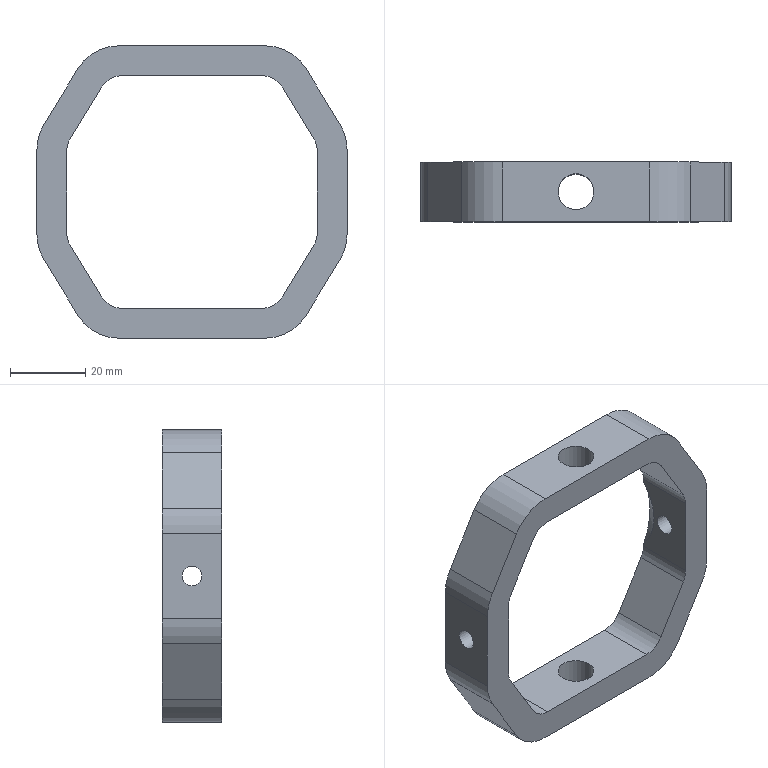Part | NX | features MG0330 trunion parts 24(gimbal) 2 | 1 solid | 40 faces | box 82.55 x 15.875 x 77.826 mm | volume 29721 mm3 | cylinder 22 | plane 18 | commonest cylinder face diameters 12.7 x8 25.4 x8 5.309 x2 9.525 x2 52.388 x2
STEP:
#1=CARTESIAN_POINT('',(33.337,-6.35,-2.654));
#2=VERTEX_POINT('',#1);
#3=CARTESIAN_POINT('',(33.337,-6.35,0.));
#4=DIRECTION('',(1.,0.,0.));
#5=DIRECTION('',(0.,0.,-1.));
#6=AXIS2_PLACEMENT_3D('',#3,#4,#5);
#7=CIRCLE('',#6,2.654);
#8=EDGE_CURVE('',#2,#2,#7,.T.);
#9=ORIENTED_EDGE('',*,*,#8,.T.);
#10=EDGE_LOOP('',(#9));
#11=FACE_BOUND('',#10,.T.);
#12=CARTESIAN_POINT('',(33.337,1.587,-10.342));
#13=VERTEX_POINT('',#12);
#14=CARTESIAN_POINT('',(33.337,1.587,-10.921));
#15=VERTEX_POINT('',#14);
#16=CARTESIAN_POINT('',(33.337,1.587,0.));
#17=DIRECTION('',(0.,0.,1.));
#18=VECTOR('',#17,1000.);
#19=LINE('',#16,#18);
#20=EDGE_CURVE('',#13,#15,#19,.F.);
#21=ORIENTED_EDGE('',*,*,#20,.T.);
#22=CARTESIAN_POINT('',(33.337,-14.287,-10.921));
#23=VERTEX_POINT('',#22);
#24=CARTESIAN_POINT('',(33.337,-14.287,-10.921));
#25=DIRECTION('',(0.,-1.,0.));
#26=VECTOR('',#25,1000.);
#27=LINE('',#24,#26);
#28=EDGE_CURVE('',#15,#23,#27,.T.);
#29=ORIENTED_EDGE('',*,*,#28,.T.);
#30=CARTESIAN_POINT('',(33.337,-14.287,10.921));
#31=VERTEX_POINT('',#30);
#32=CARTESIAN_POINT('',(33.337,-14.287,0.));
#33=DIRECTION('',(0.,0.,1.));
#34=VECTOR('',#33,1000.);
#35=LINE('',#32,#34);
#36=EDGE_CURVE('',#23,#31,#35,.T.);
#37=ORIENTED_EDGE('',*,*,#36,.T.);
#38=CARTESIAN_POINT('',(33.337,1.587,10.921));
#39=VERTEX_POINT('',#38);
#40=CARTESIAN_POINT('',(33.337,-14.287,10.921));
#41=DIRECTION('',(0.,-1.,0.));
#42=VECTOR('',#41,1000.);
#43=LINE('',#40,#42);
#44=EDGE_CURVE('',#39,#31,#43,.T.);
#45=ORIENTED_EDGE('',*,*,#44,.F.);
#46=CARTESIAN_POINT('',(33.337,1.587,10.342));
#47=VERTEX_POINT('',#46);
#48=CARTESIAN_POINT('',(33.337,1.587,0.));
#49=DIRECTION('',(0.,0.,-1.));
#50=VECTOR('',#49,1000.);
#51=LINE('',#48,#50);
#52=EDGE_CURVE('',#39,#47,#51,.T.);
#53=ORIENTED_EDGE('',*,*,#52,.T.);
#54=CARTESIAN_POINT('',(33.337,47.001,0.));
#55=DIRECTION('',(1.,0.,0.));
#56=DIRECTION('',(0.,-1.,0.));
#57=AXIS2_PLACEMENT_3D('',#54,#55,#56);
#58=ELLIPSE('',#57,49.43,26.194);
#59=EDGE_CURVE('',#13,#47,#58,.F.);
#60=ORIENTED_EDGE('',*,*,#59,.F.);
#61=EDGE_LOOP('',(#21,#29,#37,#45,#53,#60));
#62=FACE_BOUND('',#61,.T.);
#63=CARTESIAN_POINT('',(33.337,1.587,0.));
#64=DIRECTION('',(1.,0.,0.));
#65=DIRECTION('',(0.,0.,-1.));
#66=AXIS2_PLACEMENT_3D('',#63,#64,#65);
#67=PLANE('',#66);
#68=ADVANCED_FACE('',(#11,#62),#67,.F.);
#69=CARTESIAN_POINT('',(41.275,-6.35,2.654));
#70=VERTEX_POINT('',#69);
#71=CARTESIAN_POINT('',(41.275,-6.35,0.));
#72=DIRECTION('',(-1.,0.,0.));
#73=DIRECTION('',(0.,0.,1.));
#74=AXIS2_PLACEMENT_3D('',#71,#72,#73);
#75=CIRCLE('',#74,2.654);
#76=EDGE_CURVE('',#70,#70,#75,.T.);
#77=ORIENTED_EDGE('',*,*,#76,.T.);
#78=EDGE_LOOP('',(#77));
#79=FACE_BOUND('',#78,.T.);
#80=CARTESIAN_POINT('',(41.275,-14.287,11.366));
#81=VERTEX_POINT('',#80);
#82=CARTESIAN_POINT('',(41.275,-14.287,-11.366));
#83=VERTEX_POINT('',#82);
#84=CARTESIAN_POINT('',(41.275,-14.287,0.));
#85=DIRECTION('',(0.,0.,-1.));
#86=VECTOR('',#85,1000.);
#87=LINE('',#84,#86);
#88=EDGE_CURVE('',#81,#83,#87,.T.);
#89=ORIENTED_EDGE('',*,*,#88,.T.);
#90=CARTESIAN_POINT('',(41.275,1.587,-11.366));
#91=VERTEX_POINT('',#90);
#92=CARTESIAN_POINT('',(41.275,1.587,-11.366));
#93=DIRECTION('',(0.,-1.,0.));
#94=VECTOR('',#93,1000.);
#95=LINE('',#92,#94);
#96=EDGE_CURVE('',#83,#91,#95,.F.);
#97=ORIENTED_EDGE('',*,*,#96,.T.);
#98=CARTESIAN_POINT('',(41.275,1.587,11.366));
#99=VERTEX_POINT('',#98);
#100=CARTESIAN_POINT('',(41.275,1.587,0.));
#101=DIRECTION('',(0.,0.,-1.));
#102=VECTOR('',#101,1000.);
#103=LINE('',#100,#102);
#104=EDGE_CURVE('',#99,#91,#103,.T.);
#105=ORIENTED_EDGE('',*,*,#104,.F.);
#106=CARTESIAN_POINT('',(41.275,1.587,11.366));
#107=DIRECTION('',(0.,-1.,0.));
#108=VECTOR('',#107,1000.);
#109=LINE('',#106,#108);
#110=EDGE_CURVE('',#81,#99,#109,.F.);
#111=ORIENTED_EDGE('',*,*,#110,.F.);
#112=EDGE_LOOP('',(#89,#97,#105,#111));
#113=FACE_BOUND('',#112,.T.);
#114=CARTESIAN_POINT('',(41.275,1.587,0.));
#115=DIRECTION('',(-1.,0.,0.));
#116=DIRECTION('',(0.,0.,1.));
#117=AXIS2_PLACEMENT_3D('',#114,#115,#116);
#118=PLANE('',#117);
#119=ADVANCED_FACE('',(#79,#113),#118,.F.);
#120=CARTESIAN_POINT('',(39.426,1.587,-17.964));
#121=VERTEX_POINT('',#120);
#122=CARTESIAN_POINT('',(30.398,1.587,-32.811));
#123=VERTEX_POINT('',#122);
#124=CARTESIAN_POINT('',(41.275,1.587,-14.924));
#125=DIRECTION('',(-0.5196,0.,-0.8544));
#126=VECTOR('',#125,1000.);
#127=LINE('',#124,#126);
#128=EDGE_CURVE('',#121,#123,#127,.T.);
#129=ORIENTED_EDGE('',*,*,#128,.F.);
#130=CARTESIAN_POINT('',(39.426,-14.287,-17.964));
#131=VERTEX_POINT('',#130);
#132=CARTESIAN_POINT('',(39.426,1.587,-17.964));
#133=DIRECTION('',(0.,-1.,0.));
#134=VECTOR('',#133,1000.);
#135=LINE('',#132,#134);
#136=EDGE_CURVE('',#121,#131,#135,.T.);
#137=ORIENTED_EDGE('',*,*,#136,.T.);
#138=CARTESIAN_POINT('',(30.398,-14.287,-32.811));
#139=VERTEX_POINT('',#138);
#140=CARTESIAN_POINT('',(41.275,-14.287,-14.924));
#141=DIRECTION('',(-0.5196,0.,-0.8544));
#142=VECTOR('',#141,1000.);
#143=LINE('',#140,#142);
#144=EDGE_CURVE('',#131,#139,#143,.T.);
#145=ORIENTED_EDGE('',*,*,#144,.T.);
#146=CARTESIAN_POINT('',(30.398,1.587,-32.811));
#147=DIRECTION('',(0.,-1.,0.));
#148=VECTOR('',#147,1000.);
#149=LINE('',#146,#148);
#150=EDGE_CURVE('',#139,#123,#149,.F.);
#151=ORIENTED_EDGE('',*,*,#150,.T.);
#152=EDGE_LOOP('',(#129,#137,#145,#151));
#153=FACE_BOUND('',#152,.T.);
#154=CARTESIAN_POINT('',(41.275,1.587,-14.924));
#155=DIRECTION('',(-0.8544,0.,0.5196));
#156=DIRECTION('',(0.5196,0.,0.8544));
#157=AXIS2_PLACEMENT_3D('',#154,#155,#156);
#158=PLANE('',#157);
#159=ADVANCED_FACE('',(#153),#158,.F.);
#160=CARTESIAN_POINT('',(4.763,-6.35,-38.913));
#161=VERTEX_POINT('',#160);
#162=CARTESIAN_POINT('',(0.,-6.35,-38.913));
#163=DIRECTION('',(0.,0.,1.));
#164=DIRECTION('',(1.,0.,0.));
#165=AXIS2_PLACEMENT_3D('',#162,#163,#164);
#166=CIRCLE('',#165,4.763);
#167=EDGE_CURVE('',#161,#161,#166,.T.);
#168=ORIENTED_EDGE('',*,*,#167,.T.);
#169=EDGE_LOOP('',(#168));
#170=FACE_BOUND('',#169,.T.);
#171=CARTESIAN_POINT('',(19.547,1.587,-38.913));
#172=VERTEX_POINT('',#171);
#173=CARTESIAN_POINT('',(-19.547,1.587,-38.913));
#174=VERTEX_POINT('',#173);
#175=CARTESIAN_POINT('',(0.,1.587,-38.913));
#176=DIRECTION('',(-1.,0.,0.));
#177=VECTOR('',#176,1000.);
#178=LINE('',#175,#177);
#179=EDGE_CURVE('',#172,#174,#178,.T.);
#180=ORIENTED_EDGE('',*,*,#179,.F.);
#181=CARTESIAN_POINT('',(19.547,-14.287,-38.913));
#182=VERTEX_POINT('',#181);
#183=CARTESIAN_POINT('',(19.547,1.587,-38.913));
#184=DIRECTION('',(0.,-1.,0.));
#185=VECTOR('',#184,1000.);
#186=LINE('',#183,#185);
#187=EDGE_CURVE('',#172,#182,#186,.T.);
#188=ORIENTED_EDGE('',*,*,#187,.T.);
#189=CARTESIAN_POINT('',(-19.547,-14.287,-38.913));
#190=VERTEX_POINT('',#189);
#191=CARTESIAN_POINT('',(0.,-14.287,-38.913));
#192=DIRECTION('',(-1.,0.,0.));
#193=VECTOR('',#192,1000.);
#194=LINE('',#191,#193);
#195=EDGE_CURVE('',#182,#190,#194,.T.);
#196=ORIENTED_EDGE('',*,*,#195,.T.);
#197=CARTESIAN_POINT('',(-19.547,1.587,-38.913));
#198=DIRECTION('',(0.,-1.,0.));
#199=VECTOR('',#198,1000.);
#200=LINE('',#197,#199);
#201=EDGE_CURVE('',#174,#190,#200,.T.);
#202=ORIENTED_EDGE('',*,*,#201,.F.);
#203=EDGE_LOOP('',(#180,#188,#196,#202));
#204=FACE_BOUND('',#203,.T.);
#205=CARTESIAN_POINT('',(0.,1.587,-38.913));
#206=DIRECTION('',(0.,0.,1.));
#207=DIRECTION('',(1.,0.,0.));
#208=AXIS2_PLACEMENT_3D('',#205,#206,#207);
#209=PLANE('',#208);
#210=ADVANCED_FACE('',(#170,#204),#209,.F.);
#211=CARTESIAN_POINT('',(-4.763,-6.35,-30.975));
#212=VERTEX_POINT('',#211);
#213=CARTESIAN_POINT('',(0.,-6.35,-30.975));
#214=DIRECTION('',(0.,0.,-1.));
#215=DIRECTION('',(-1.,0.,0.));
#216=AXIS2_PLACEMENT_3D('',#213,#214,#215);
#217=CIRCLE('',#216,4.763);
#218=EDGE_CURVE('',#212,#212,#217,.T.);
#219=ORIENTED_EDGE('',*,*,#218,.T.);
#220=EDGE_LOOP('',(#219));
#221=FACE_BOUND('',#220,.T.);
#222=CARTESIAN_POINT('',(-18.654,-14.287,-30.975));
#223=VERTEX_POINT('',#222);
#224=CARTESIAN_POINT('',(18.654,-14.287,-30.975));
#225=VERTEX_POINT('',#224);
#226=CARTESIAN_POINT('',(0.,-14.287,-30.975));
#227=DIRECTION('',(1.,0.,0.));
#228=VECTOR('',#227,1000.);
#229=LINE('',#226,#228);
#230=EDGE_CURVE('',#223,#225,#229,.T.);
#231=ORIENTED_EDGE('',*,*,#230,.T.);
#232=CARTESIAN_POINT('',(18.654,1.587,-30.975));
#233=VERTEX_POINT('',#232);
#234=CARTESIAN_POINT('',(18.654,1.587,-30.975));
#235=DIRECTION('',(0.,-1.,0.));
#236=VECTOR('',#235,1000.);
#237=LINE('',#234,#236);
#238=EDGE_CURVE('',#225,#233,#237,.F.);
#239=ORIENTED_EDGE('',*,*,#238,.T.);
#240=CARTESIAN_POINT('',(-18.654,1.587,-30.975));
#241=VERTEX_POINT('',#240);
#242=CARTESIAN_POINT('',(0.,1.587,-30.975));
#243=DIRECTION('',(1.,0.,0.));
#244=VECTOR('',#243,1000.);
#245=LINE('',#242,#244);
#246=EDGE_CURVE('',#241,#233,#245,.T.);
#247=ORIENTED_EDGE('',*,*,#246,.F.);
#248=CARTESIAN_POINT('',(-18.654,1.587,-30.975));
#249=DIRECTION('',(0.,-1.,0.));
#250=VECTOR('',#249,1000.);
#251=LINE('',#248,#250);
#252=EDGE_CURVE('',#223,#241,#251,.F.);
#253=ORIENTED_EDGE('',*,*,#252,.F.);
#254=EDGE_LOOP('',(#231,#239,#247,#253));
#255=FACE_BOUND('',#254,.T.);
#256=CARTESIAN_POINT('',(0.,1.587,-30.975));
#257=DIRECTION('',(0.,0.,-1.));
#258=DIRECTION('',(-1.,0.,0.));
#259=AXIS2_PLACEMENT_3D('',#256,#257,#258);
#260=PLANE('',#259);
#261=ADVANCED_FACE('',(#221,#255),#260,.F.);
#262=CARTESIAN_POINT('',(24.08,1.587,-27.924));
#263=VERTEX_POINT('',#262);
#264=CARTESIAN_POINT('',(32.413,1.587,-14.22));
#265=VERTEX_POINT('',#264);
#266=CARTESIAN_POINT('',(33.337,1.587,-12.7));
#267=DIRECTION('',(0.5196,0.,0.8544));
#268=VECTOR('',#267,1000.);
#269=LINE('',#266,#268);
#270=EDGE_CURVE('',#263,#265,#269,.T.);
#271=ORIENTED_EDGE('',*,*,#270,.F.);
#272=CARTESIAN_POINT('',(24.08,-14.287,-27.924));
#273=VERTEX_POINT('',#272);
#274=CARTESIAN_POINT('',(24.08,-14.287,-27.924));
#275=DIRECTION('',(0.,-1.,0.));
#276=VECTOR('',#275,1000.);
#277=LINE('',#274,#276);
#278=EDGE_CURVE('',#263,#273,#277,.T.);
#279=ORIENTED_EDGE('',*,*,#278,.T.);
#280=CARTESIAN_POINT('',(32.413,-14.287,-14.22));
#281=VERTEX_POINT('',#280);
#282=CARTESIAN_POINT('',(33.337,-14.287,-12.7));
#283=DIRECTION('',(0.5196,0.,0.8544));
#284=VECTOR('',#283,1000.);
#285=LINE('',#282,#284);
#286=EDGE_CURVE('',#273,#281,#285,.T.);
#287=ORIENTED_EDGE('',*,*,#286,.T.);
#288=CARTESIAN_POINT('',(32.413,1.587,-14.22));
#289=DIRECTION('',(0.,-1.,0.));
#290=VECTOR('',#289,1000.);
#291=LINE('',#288,#290);
#292=EDGE_CURVE('',#281,#265,#291,.F.);
#293=ORIENTED_EDGE('',*,*,#292,.T.);
#294=EDGE_LOOP('',(#271,#279,#287,#293));
#295=FACE_BOUND('',#294,.T.);
#296=CARTESIAN_POINT('',(33.337,1.587,-12.7));
#297=DIRECTION('',(0.8544,0.,-0.5196));
#298=DIRECTION('',(-0.5196,0.,-0.8544));
#299=AXIS2_PLACEMENT_3D('',#296,#297,#298);
#300=PLANE('',#299);
#301=ADVANCED_FACE('',(#295),#300,.F.);
#302=CARTESIAN_POINT('',(-24.08,1.587,-27.924));
#303=VERTEX_POINT('',#302);
#304=CARTESIAN_POINT('',(-18.654,1.587,-24.625));
#305=DIRECTION('',(0.,1.,0.));
#306=DIRECTION('',(0.,0.,-1.));
#307=AXIS2_PLACEMENT_3D('',#304,#305,#306);
#308=CIRCLE('',#307,6.35);
#309=EDGE_CURVE('',#241,#303,#308,.T.);
#310=ORIENTED_EDGE('',*,*,#309,.F.);
#311=ORIENTED_EDGE('',*,*,#246,.T.);
#312=CARTESIAN_POINT('',(18.654,1.587,-24.625));
#313=DIRECTION('',(0.,-1.,0.));
#314=DIRECTION('',(0.,0.,-1.));
#315=AXIS2_PLACEMENT_3D('',#312,#313,#314);
#316=CIRCLE('',#315,6.35);
#317=EDGE_CURVE('',#233,#263,#316,.T.);
#318=ORIENTED_EDGE('',*,*,#317,.T.);
#319=ORIENTED_EDGE('',*,*,#270,.T.);
#320=CARTESIAN_POINT('',(26.988,1.587,-10.921));
#321=DIRECTION('',(0.,-1.,0.));
#322=DIRECTION('',(0.,0.,-1.));
#323=AXIS2_PLACEMENT_3D('',#320,#321,#322);
#324=CIRCLE('',#323,6.35);
#325=EDGE_CURVE('',#265,#15,#324,.T.);
#326=ORIENTED_EDGE('',*,*,#325,.T.);
#327=ORIENTED_EDGE('',*,*,#20,.F.);
#328=CARTESIAN_POINT('',(4.96,1.587,0.));
#329=DIRECTION('',(0.,-1.,0.));
#330=DIRECTION('',(-1.,0.,0.));
#331=AXIS2_PLACEMENT_3D('',#328,#329,#330);
#332=ELLIPSE('',#331,30.887,26.194);
#333=EDGE_CURVE('',#47,#13,#332,.F.);
#334=ORIENTED_EDGE('',*,*,#333,.F.);
#335=ORIENTED_EDGE('',*,*,#52,.F.);
#336=CARTESIAN_POINT('',(32.413,1.587,14.22));
#337=VERTEX_POINT('',#336);
#338=CARTESIAN_POINT('',(26.988,1.587,10.921));
#339=DIRECTION('',(0.,1.,0.));
#340=DIRECTION('',(0.,0.,1.));
#341=AXIS2_PLACEMENT_3D('',#338,#339,#340);
#342=CIRCLE('',#341,6.35);
#343=EDGE_CURVE('',#337,#39,#342,.T.);
#344=ORIENTED_EDGE('',*,*,#343,.F.);
#345=CARTESIAN_POINT('',(24.08,1.587,27.924));
#346=VERTEX_POINT('',#345);
#347=CARTESIAN_POINT('',(33.337,1.587,12.7));
#348=DIRECTION('',(0.5196,0.,-0.8544));
#349=VECTOR('',#348,1000.);
#350=LINE('',#347,#349);
#351=EDGE_CURVE('',#346,#337,#350,.T.);
#352=ORIENTED_EDGE('',*,*,#351,.F.);
#353=CARTESIAN_POINT('',(18.654,1.587,30.975));
#354=VERTEX_POINT('',#353);
#355=CARTESIAN_POINT('',(18.654,1.587,24.625));
#356=DIRECTION('',(0.,1.,0.));
#357=DIRECTION('',(0.,0.,1.));
#358=AXIS2_PLACEMENT_3D('',#355,#356,#357);
#359=CIRCLE('',#358,6.35);
#360=EDGE_CURVE('',#354,#346,#359,.T.);
#361=ORIENTED_EDGE('',*,*,#360,.F.);
#362=CARTESIAN_POINT('',(-18.654,1.587,30.975));
#363=VERTEX_POINT('',#362);
#364=CARTESIAN_POINT('',(0.,1.587,30.975));
#365=DIRECTION('',(1.,0.,0.));
#366=VECTOR('',#365,1000.);
#367=LINE('',#364,#366);
#368=EDGE_CURVE('',#363,#354,#367,.T.);
#369=ORIENTED_EDGE('',*,*,#368,.F.);
#370=CARTESIAN_POINT('',(-24.08,1.587,27.924));
#371=VERTEX_POINT('',#370);
#372=CARTESIAN_POINT('',(-18.654,1.587,24.625));
#373=DIRECTION('',(0.,-1.,0.));
#374=DIRECTION('',(0.,0.,1.));
#375=AXIS2_PLACEMENT_3D('',#372,#373,#374);
#376=CIRCLE('',#375,6.35);
#377=EDGE_CURVE('',#363,#371,#376,.T.);
#378=ORIENTED_EDGE('',*,*,#377,.T.);
#379=CARTESIAN_POINT('',(-32.413,1.587,14.22));
#380=VERTEX_POINT('',#379);
#381=CARTESIAN_POINT('',(-33.337,1.587,12.7));
#382=DIRECTION('',(-0.5196,0.,-0.8544));
#383=VECTOR('',#382,1000.);
#384=LINE('',#381,#383);
#385=EDGE_CURVE('',#371,#380,#384,.T.);
#386=ORIENTED_EDGE('',*,*,#385,.T.);
#387=CARTESIAN_POINT('',(-33.337,1.587,10.921));
#388=VERTEX_POINT('',#387);
#389=CARTESIAN_POINT('',(-26.988,1.587,10.921));
#390=DIRECTION('',(0.,-1.,0.));
#391=DIRECTION('',(0.,0.,1.));
#392=AXIS2_PLACEMENT_3D('',#389,#390,#391);
#393=CIRCLE('',#392,6.35);
#394=EDGE_CURVE('',#380,#388,#393,.T.);
#395=ORIENTED_EDGE('',*,*,#394,.T.);
#396=CARTESIAN_POINT('',(-33.337,1.587,10.342));
#397=VERTEX_POINT('',#396);
#398=CARTESIAN_POINT('',(-33.337,1.587,0.));
#399=DIRECTION('',(0.,0.,-1.));
#400=VECTOR('',#399,1000.);
#401=LINE('',#398,#400);
#402=EDGE_CURVE('',#388,#397,#401,.T.);
#403=ORIENTED_EDGE('',*,*,#402,.T.);
#404=CARTESIAN_POINT('',(-33.337,1.587,-10.342));
#405=VERTEX_POINT('',#404);
#406=CARTESIAN_POINT('',(-4.96,1.587,0.));
#407=DIRECTION('',(0.,1.,0.));
#408=DIRECTION('',(1.,0.,0.));
#409=AXIS2_PLACEMENT_3D('',#406,#407,#408);
#410=ELLIPSE('',#409,30.887,26.194);
#411=EDGE_CURVE('',#397,#405,#410,.F.);
#412=ORIENTED_EDGE('',*,*,#411,.T.);
#413=CARTESIAN_POINT('',(-33.337,1.587,-10.921));
#414=VERTEX_POINT('',#413);
#415=CARTESIAN_POINT('',(-33.337,1.587,0.));
#416=DIRECTION('',(0.,0.,1.));
#417=VECTOR('',#416,1000.);
#418=LINE('',#415,#417);
#419=EDGE_CURVE('',#405,#414,#418,.F.);
#420=ORIENTED_EDGE('',*,*,#419,.T.);
#421=CARTESIAN_POINT('',(-32.413,1.587,-14.22));
#422=VERTEX_POINT('',#421);
#423=CARTESIAN_POINT('',(-26.988,1.587,-10.921));
#424=DIRECTION('',(0.,1.,0.));
#425=DIRECTION('',(0.,0.,-1.));
#426=AXIS2_PLACEMENT_3D('',#423,#424,#425);
#427=CIRCLE('',#426,6.35);
#428=EDGE_CURVE('',#422,#414,#427,.T.);
#429=ORIENTED_EDGE('',*,*,#428,.F.);
#430=CARTESIAN_POINT('',(-33.337,1.587,-12.7));
#431=DIRECTION('',(-0.5196,0.,0.8544));
#432=VECTOR('',#431,1000.);
#433=LINE('',#430,#432);
#434=EDGE_CURVE('',#303,#422,#433,.T.);
#435=ORIENTED_EDGE('',*,*,#434,.F.);
#436=EDGE_LOOP('',(#310,#311,#318,#319,#326,#327,#334,#335,#344,#352,#361,#369,#378,#386,#395,#403,#412,#420,#429,#435));
#437=FACE_BOUND('',#436,.T.);
#438=ORIENTED_EDGE('',*,*,#104,.T.);
#439=CARTESIAN_POINT('',(28.575,1.587,-11.366));
#440=DIRECTION('',(0.,-1.,0.));
#441=DIRECTION('',(0.,0.,-1.));
#442=AXIS2_PLACEMENT_3D('',#439,#440,#441);
#443=CIRCLE('',#442,12.7);
#444=EDGE_CURVE('',#91,#121,#443,.F.);
#445=ORIENTED_EDGE('',*,*,#444,.T.);
#446=ORIENTED_EDGE('',*,*,#128,.T.);
#447=CARTESIAN_POINT('',(19.547,1.587,-26.213));
#448=DIRECTION('',(0.,-1.,0.));
#449=DIRECTION('',(0.,0.,-1.));
#450=AXIS2_PLACEMENT_3D('',#447,#448,#449);
#451=CIRCLE('',#450,12.7);
#452=EDGE_CURVE('',#123,#172,#451,.F.);
#453=ORIENTED_EDGE('',*,*,#452,.T.);
#454=ORIENTED_EDGE('',*,*,#179,.T.);
#455=CARTESIAN_POINT('',(-30.398,1.587,-32.811));
#456=VERTEX_POINT('',#455);
#457=CARTESIAN_POINT('',(-19.547,1.587,-26.213));
#458=DIRECTION('',(0.,1.,0.));
#459=DIRECTION('',(0.,0.,-1.));
#460=AXIS2_PLACEMENT_3D('',#457,#458,#459);
#461=CIRCLE('',#460,12.7);
#462=EDGE_CURVE('',#456,#174,#461,.F.);
#463=ORIENTED_EDGE('',*,*,#462,.F.);
#464=CARTESIAN_POINT('',(-39.426,1.587,-17.964));
#465=VERTEX_POINT('',#464);
#466=CARTESIAN_POINT('',(-41.275,1.587,-14.924));
#467=DIRECTION('',(0.5196,0.,-0.8544));
#468=VECTOR('',#467,1000.);
#469=LINE('',#466,#468);
#470=EDGE_CURVE('',#465,#456,#469,.T.);
#471=ORIENTED_EDGE('',*,*,#470,.F.);
#472=CARTESIAN_POINT('',(-41.275,1.587,-11.366));
#473=VERTEX_POINT('',#472);
#474=CARTESIAN_POINT('',(-28.575,1.587,-11.366));
#475=DIRECTION('',(0.,1.,0.));
#476=DIRECTION('',(0.,0.,-1.));
#477=AXIS2_PLACEMENT_3D('',#474,#475,#476);
#478=CIRCLE('',#477,12.7);
#479=EDGE_CURVE('',#473,#465,#478,.F.);
#480=ORIENTED_EDGE('',*,*,#479,.F.);
#481=CARTESIAN_POINT('',(-41.275,1.587,11.366));
#482=VERTEX_POINT('',#481);
#483=CARTESIAN_POINT('',(-41.275,1.587,0.));
#484=DIRECTION('',(0.,0.,-1.));
#485=VECTOR('',#484,1000.);
#486=LINE('',#483,#485);
#487=EDGE_CURVE('',#482,#473,#486,.T.);
#488=ORIENTED_EDGE('',*,*,#487,.F.);
#489=CARTESIAN_POINT('',(-39.426,1.587,17.964));
#490=VERTEX_POINT('',#489);
#491=CARTESIAN_POINT('',(-28.575,1.587,11.366));
#492=DIRECTION('',(0.,-1.,0.));
#493=DIRECTION('',(0.,0.,1.));
#494=AXIS2_PLACEMENT_3D('',#491,#492,#493);
#495=CIRCLE('',#494,12.7);
#496=EDGE_CURVE('',#482,#490,#495,.F.);
#497=ORIENTED_EDGE('',*,*,#496,.T.);
#498=CARTESIAN_POINT('',(-30.398,1.587,32.811));
#499=VERTEX_POINT('',#498);
#500=CARTESIAN_POINT('',(-41.275,1.587,14.924));
#501=DIRECTION('',(0.5196,0.,0.8544));
#502=VECTOR('',#501,1000.);
#503=LINE('',#500,#502);
#504=EDGE_CURVE('',#490,#499,#503,.T.);
#505=ORIENTED_EDGE('',*,*,#504,.T.);
#506=CARTESIAN_POINT('',(-19.547,1.587,38.913));
#507=VERTEX_POINT('',#506);
#508=CARTESIAN_POINT('',(-19.547,1.587,26.213));
#509=DIRECTION('',(0.,-1.,0.));
#510=DIRECTION('',(0.,0.,1.));
#511=AXIS2_PLACEMENT_3D('',#508,#509,#510);
#512=CIRCLE('',#511,12.7);
#513=EDGE_CURVE('',#499,#507,#512,.F.);
#514=ORIENTED_EDGE('',*,*,#513,.T.);
#515=CARTESIAN_POINT('',(19.547,1.587,38.913));
#516=VERTEX_POINT('',#515);
#517=CARTESIAN_POINT('',(0.,1.587,38.913));
#518=DIRECTION('',(-1.,0.,0.));
#519=VECTOR('',#518,1000.);
#520=LINE('',#517,#519);
#521=EDGE_CURVE('',#516,#507,#520,.T.);
#522=ORIENTED_EDGE('',*,*,#521,.F.);
#523=CARTESIAN_POINT('',(30.398,1.587,32.811));
#524=VERTEX_POINT('',#523);
#525=CARTESIAN_POINT('',(19.547,1.587,26.213));
#526=DIRECTION('',(0.,1.,0.));
#527=DIRECTION('',(0.,0.,1.));
#528=AXIS2_PLACEMENT_3D('',#525,#526,#527);
#529=CIRCLE('',#528,12.7);
#530=EDGE_CURVE('',#524,#516,#529,.F.);
#531=ORIENTED_EDGE('',*,*,#530,.F.);
#532=CARTESIAN_POINT('',(39.426,1.587,17.964));
#533=VERTEX_POINT('',#532);
#534=CARTESIAN_POINT('',(41.275,1.587,14.924));
#535=DIRECTION('',(-0.5196,0.,0.8544));
#536=VECTOR('',#535,1000.);
#537=LINE('',#534,#536);
#538=EDGE_CURVE('',#533,#524,#537,.T.);
#539=ORIENTED_EDGE('',*,*,#538,.F.);
#540=CARTESIAN_POINT('',(28.575,1.587,11.366));
#541=DIRECTION('',(0.,1.,0.));
#542=DIRECTION('',(0.,0.,1.));
#543=AXIS2_PLACEMENT_3D('',#540,#541,#542);
#544=CIRCLE('',#543,12.7);
#545=EDGE_CURVE('',#99,#533,#544,.F.);
#546=ORIENTED_EDGE('',*,*,#545,.F.);
#547=EDGE_LOOP('',(#438,#445,#446,#453,#454,#463,#471,#480,#488,#497,#505,#514,#522,#531,#539,#546));
#548=FACE_BOUND('',#547,.T.);
#549=CARTESIAN_POINT('',(33.337,1.587,-38.913));
#550=DIRECTION('',(0.,-1.,0.));
#551=DIRECTION('',(0.,0.,-1.));
#552=AXIS2_PLACEMENT_3D('',#549,#550,#551);
#553=PLANE('',#552);
#554=ADVANCED_FACE('',(#437,#548),#553,.F.);
#555=ORIENTED_EDGE('',*,*,#230,.F.);
#556=CARTESIAN_POINT('',(-24.08,-14.287,-27.924));
#557=VERTEX_POINT('',#556);
#558=CARTESIAN_POINT('',(-18.654,-14.287,-24.625));
#559=DIRECTION('',(0.,1.,0.));
#560=DIRECTION('',(0.,0.,-1.));
#561=AXIS2_PLACEMENT_3D('',#558,#559,#560);
#562=CIRCLE('',#561,6.35);
#563=EDGE_CURVE('',#557,#223,#562,.F.);
#564=ORIENTED_EDGE('',*,*,#563,.F.);
#565=CARTESIAN_POINT('',(-32.413,-14.287,-14.22));
#566=VERTEX_POINT('',#565);
#567=CARTESIAN_POINT('',(-33.337,-14.287,-12.7));
#568=DIRECTION('',(-0.5196,0.,0.8544));
#569=VECTOR('',#568,1000.);
#570=LINE('',#567,#569);
#571=EDGE_CURVE('',#557,#566,#570,.T.);
#572=ORIENTED_EDGE('',*,*,#571,.T.);
#573=CARTESIAN_POINT('',(-33.337,-14.287,-10.921));
#574=VERTEX_POINT('',#573);
#575=CARTESIAN_POINT('',(-26.988,-14.287,-10.921));
#576=DIRECTION('',(0.,1.,0.));
#577=DIRECTION('',(0.,0.,-1.));
#578=AXIS2_PLACEMENT_3D('',#575,#576,#577);
#579=CIRCLE('',#578,6.35);
#580=EDGE_CURVE('',#574,#566,#579,.F.);
#581=ORIENTED_EDGE('',*,*,#580,.F.);
#582=CARTESIAN_POINT('',(-33.337,-14.287,10.921));
#583=VERTEX_POINT('',#582);
#584=CARTESIAN_POINT('',(-33.337,-14.287,0.));
#585=DIRECTION('',(0.,0.,1.));
#586=VECTOR('',#585,1000.);
#587=LINE('',#584,#586);
#588=EDGE_CURVE('',#574,#583,#587,.T.);
#589=ORIENTED_EDGE('',*,*,#588,.T.);
#590=CARTESIAN_POINT('',(-32.413,-14.287,14.22));
#591=VERTEX_POINT('',#590);
#592=CARTESIAN_POINT('',(-26.988,-14.287,10.921));
#593=DIRECTION('',(0.,-1.,0.));
#594=DIRECTION('',(0.,0.,1.));
#595=AXIS2_PLACEMENT_3D('',#592,#593,#594);
#596=CIRCLE('',#595,6.35);
#597=EDGE_CURVE('',#583,#591,#596,.F.);
#598=ORIENTED_EDGE('',*,*,#597,.T.);
#599=CARTESIAN_POINT('',(-24.08,-14.287,27.924));
#600=VERTEX_POINT('',#599);
#601=CARTESIAN_POINT('',(-33.337,-14.287,12.7));
#602=DIRECTION('',(-0.5196,0.,-0.8544));
#603=VECTOR('',#602,1000.);
#604=LINE('',#601,#603);
#605=EDGE_CURVE('',#600,#591,#604,.T.);
#606=ORIENTED_EDGE('',*,*,#605,.F.);
#607=CARTESIAN_POINT('',(-18.654,-14.287,30.975));
#608=VERTEX_POINT('',#607);
#609=CARTESIAN_POINT('',(-18.654,-14.287,24.625));
#610=DIRECTION('',(0.,-1.,0.));
#611=DIRECTION('',(0.,0.,1.));
#612=AXIS2_PLACEMENT_3D('',#609,#610,#611);
#613=CIRCLE('',#612,6.35);
#614=EDGE_CURVE('',#600,#608,#613,.F.);
#615=ORIENTED_EDGE('',*,*,#614,.T.);
#616=CARTESIAN_POINT('',(18.654,-14.287,30.975));
#617=VERTEX_POINT('',#616);
#618=CARTESIAN_POINT('',(0.,-14.287,30.975));
#619=DIRECTION('',(1.,0.,0.));
#620=VECTOR('',#619,1000.);
#621=LINE('',#618,#620);
#622=EDGE_CURVE('',#608,#617,#621,.T.);
#623=ORIENTED_EDGE('',*,*,#622,.T.);
#624=CARTESIAN_POINT('',(24.08,-14.287,27.924));
#625=VERTEX_POINT('',#624);
#626=CARTESIAN_POINT('',(18.654,-14.287,24.625));
#627=DIRECTION('',(0.,1.,0.));
#628=DIRECTION('',(0.,0.,1.));
#629=AXIS2_PLACEMENT_3D('',#626,#627,#628);
#630=CIRCLE('',#629,6.35);
#631=EDGE_CURVE('',#625,#617,#630,.F.);
#632=ORIENTED_EDGE('',*,*,#631,.F.);
#633=CARTESIAN_POINT('',(32.413,-14.287,14.22));
#634=VERTEX_POINT('',#633);
#635=CARTESIAN_POINT('',(33.337,-14.287,12.7));
#636=DIRECTION('',(0.5196,0.,-0.8544));
#637=VECTOR('',#636,1000.);
#638=LINE('',#635,#637);
#639=EDGE_CURVE('',#625,#634,#638,.T.);
#640=ORIENTED_EDGE('',*,*,#639,.T.);
#641=CARTESIAN_POINT('',(26.988,-14.287,10.921));
#642=DIRECTION('',(0.,1.,0.));
#643=DIRECTION('',(0.,0.,1.));
#644=AXIS2_PLACEMENT_3D('',#641,#642,#643);
#645=CIRCLE('',#644,6.35);
#646=EDGE_CURVE('',#31,#634,#645,.F.);
#647=ORIENTED_EDGE('',*,*,#646,.F.);
#648=ORIENTED_EDGE('',*,*,#36,.F.);
#649=CARTESIAN_POINT('',(26.988,-14.287,-10.921));
#650=DIRECTION('',(0.,-1.,0.));
#651=DIRECTION('',(0.,0.,-1.));
#652=AXIS2_PLACEMENT_3D('',#649,#650,#651);
#653=CIRCLE('',#652,6.35);
#654=EDGE_CURVE('',#23,#281,#653,.F.);
#655=ORIENTED_EDGE('',*,*,#654,.T.);
#656=ORIENTED_EDGE('',*,*,#286,.F.);
#657=CARTESIAN_POINT('',(18.654,-14.287,-24.625));
#658=DIRECTION('',(0.,-1.,0.));
#659=DIRECTION('',(0.,0.,-1.));
#660=AXIS2_PLACEMENT_3D('',#657,#658,#659);
#661=CIRCLE('',#660,6.35);
#662=EDGE_CURVE('',#273,#225,#661,.F.);
#663=ORIENTED_EDGE('',*,*,#662,.T.);
#664=EDGE_LOOP('',(#555,#564,#572,#581,#589,#598,#606,#615,#623,#632,#640,#647,#648,#655,#656,#663));
#665=FACE_BOUND('',#664,.T.);
#666=ORIENTED_EDGE('',*,*,#144,.F.);
#667=CARTESIAN_POINT('',(28.575,-14.287,-11.366));
#668=DIRECTION('',(0.,-1.,0.));
#669=DIRECTION('',(0.,0.,-1.));
#670=AXIS2_PLACEMENT_3D('',#667,#668,#669);
#671=CIRCLE('',#670,12.7);
#672=EDGE_CURVE('',#131,#83,#671,.T.);
#673=ORIENTED_EDGE('',*,*,#672,.T.);
#674=ORIENTED_EDGE('',*,*,#88,.F.);
#675=CARTESIAN_POINT('',(39.426,-14.287,17.964));
#676=VERTEX_POINT('',#675);
#677=CARTESIAN_POINT('',(28.575,-14.287,11.366));
#678=DIRECTION('',(0.,1.,0.));
#679=DIRECTION('',(0.,0.,1.));
#680=AXIS2_PLACEMENT_3D('',#677,#678,#679);
#681=CIRCLE('',#680,12.7);
#682=EDGE_CURVE('',#676,#81,#681,.T.);
#683=ORIENTED_EDGE('',*,*,#682,.F.);
#684=CARTESIAN_POINT('',(30.398,-14.287,32.811));
#685=VERTEX_POINT('',#684);
#686=CARTESIAN_POINT('',(41.275,-14.287,14.924));
#687=DIRECTION('',(-0.5196,0.,0.8544));
#688=VECTOR('',#687,1000.);
#689=LINE('',#686,#688);
#690=EDGE_CURVE('',#676,#685,#689,.T.);
#691=ORIENTED_EDGE('',*,*,#690,.T.);
#692=CARTESIAN_POINT('',(19.547,-14.287,38.913));
#693=VERTEX_POINT('',#692);
#694=CARTESIAN_POINT('',(19.547,-14.287,26.213));
#695=DIRECTION('',(0.,1.,0.));
#696=DIRECTION('',(0.,0.,1.));
#697=AXIS2_PLACEMENT_3D('',#694,#695,#696);
#698=CIRCLE('',#697,12.7);
#699=EDGE_CURVE('',#693,#685,#698,.T.);
#700=ORIENTED_EDGE('',*,*,#699,.F.);
#701=CARTESIAN_POINT('',(-19.547,-14.287,38.913));
#702=VERTEX_POINT('',#701);
#703=CARTESIAN_POINT('',(0.,-14.287,38.913));
#704=DIRECTION('',(-1.,0.,0.));
#705=VECTOR('',#704,1000.);
#706=LINE('',#703,#705);
#707=EDGE_CURVE('',#693,#702,#706,.T.);
#708=ORIENTED_EDGE('',*,*,#707,.T.);
#709=CARTESIAN_POINT('',(-30.398,-14.287,32.811));
#710=VERTEX_POINT('',#709);
#711=CARTESIAN_POINT('',(-19.547,-14.287,26.213));
#712=DIRECTION('',(0.,-1.,0.));
#713=DIRECTION('',(0.,0.,1.));
#714=AXIS2_PLACEMENT_3D('',#711,#712,#713);
#715=CIRCLE('',#714,12.7);
#716=EDGE_CURVE('',#702,#710,#715,.T.);
#717=ORIENTED_EDGE('',*,*,#716,.T.);
#718=CARTESIAN_POINT('',(-39.426,-14.287,17.964));
#719=VERTEX_POINT('',#718);
#720=CARTESIAN_POINT('',(-41.275,-14.287,14.924));
#721=DIRECTION('',(0.5196,0.,0.8544));
#722=VECTOR('',#721,1000.);
#723=LINE('',#720,#722);
#724=EDGE_CURVE('',#719,#710,#723,.T.);
#725=ORIENTED_EDGE('',*,*,#724,.F.);
#726=CARTESIAN_POINT('',(-41.275,-14.287,11.366));
#727=VERTEX_POINT('',#726);
#728=CARTESIAN_POINT('',(-28.575,-14.287,11.366));
#729=DIRECTION('',(0.,-1.,0.));
#730=DIRECTION('',(0.,0.,1.));
#731=AXIS2_PLACEMENT_3D('',#728,#729,#730);
#732=CIRCLE('',#731,12.7);
#733=EDGE_CURVE('',#719,#727,#732,.T.);
#734=ORIENTED_EDGE('',*,*,#733,.T.);
#735=CARTESIAN_POINT('',(-41.275,-14.287,-11.366));
#736=VERTEX_POINT('',#735);
#737=CARTESIAN_POINT('',(-41.275,-14.287,0.));
#738=DIRECTION('',(0.,0.,-1.));
#739=VECTOR('',#738,1000.);
#740=LINE('',#737,#739);
#741=EDGE_CURVE('',#727,#736,#740,.T.);
#742=ORIENTED_EDGE('',*,*,#741,.T.);
#743=CARTESIAN_POINT('',(-39.426,-14.287,-17.964));
#744=VERTEX_POINT('',#743);
#745=CARTESIAN_POINT('',(-28.575,-14.287,-11.366));
#746=DIRECTION('',(0.,1.,0.));
#747=DIRECTION('',(0.,0.,-1.));
#748=AXIS2_PLACEMENT_3D('',#745,#746,#747);
#749=CIRCLE('',#748,12.7);
#750=EDGE_CURVE('',#744,#736,#749,.T.);
#751=ORIENTED_EDGE('',*,*,#750,.F.);
#752=CARTESIAN_POINT('',(-30.398,-14.287,-32.811));
#753=VERTEX_POINT('',#752);
#754=CARTESIAN_POINT('',(-41.275,-14.287,-14.924));
#755=DIRECTION('',(0.5196,0.,-0.8544));
#756=VECTOR('',#755,1000.);
#757=LINE('',#754,#756);
#758=EDGE_CURVE('',#744,#753,#757,.T.);
#759=ORIENTED_EDGE('',*,*,#758,.T.);
#760=CARTESIAN_POINT('',(-19.547,-14.287,-26.213));
#761=DIRECTION('',(0.,1.,0.));
#762=DIRECTION('',(0.,0.,-1.));
#763=AXIS2_PLACEMENT_3D('',#760,#761,#762);
#764=CIRCLE('',#763,12.7);
#765=EDGE_CURVE('',#190,#753,#764,.T.);
#766=ORIENTED_EDGE('',*,*,#765,.F.);
#767=ORIENTED_EDGE('',*,*,#195,.F.);
#768=CARTESIAN_POINT('',(19.547,-14.287,-26.213));
#769=DIRECTION('',(0.,-1.,0.));
#770=DIRECTION('',(0.,0.,-1.));
#771=AXIS2_PLACEMENT_3D('',#768,#769,#770);
#772=CIRCLE('',#771,12.7);
#773=EDGE_CURVE('',#182,#139,#772,.T.);
#774=ORIENTED_EDGE('',*,*,#773,.T.);
#775=EDGE_LOOP('',(#666,#673,#674,#683,#691,#700,#708,#717,#725,#734,#742,#751,#759,#766,#767,#774));
#776=FACE_BOUND('',#775,.T.);
#777=CARTESIAN_POINT('',(33.337,-14.287,-38.913));
#778=DIRECTION('',(0.,-1.,0.));
#779=DIRECTION('',(0.,0.,-1.));
#780=AXIS2_PLACEMENT_3D('',#777,#778,#779);
#781=PLANE('',#780);
#782=ADVANCED_FACE('',(#665,#776),#781,.T.);
#783=ORIENTED_EDGE('',*,*,#59,.T.);
#784=ORIENTED_EDGE('',*,*,#333,.T.);
#785=EDGE_LOOP('',(#783,#784));
#786=FACE_BOUND('',#785,.T.);
#787=CARTESIAN_POINT('',(26.92,36.731,0.));
#788=DIRECTION('',(-0.5299,-0.848,0.));
#789=DIRECTION('',(0.848,-0.5299,0.));
#790=AXIS2_PLACEMENT_3D('',#787,#788,#789);
#791=CYLINDRICAL_SURFACE('',#790,26.194);
#792=ADVANCED_FACE('',(#786),#791,.F.);
#793=ORIENTED_EDGE('',*,*,#317,.F.);
#794=ORIENTED_EDGE('',*,*,#238,.F.);
#795=ORIENTED_EDGE('',*,*,#662,.F.);
#796=ORIENTED_EDGE('',*,*,#278,.F.);
#797=EDGE_LOOP('',(#793,#794,#795,#796));
#798=FACE_BOUND('',#797,.T.);
#799=CARTESIAN_POINT('',(18.654,1.587,-24.625));
#800=DIRECTION('',(0.,1.,0.));
#801=DIRECTION('',(0.,0.,1.));
#802=AXIS2_PLACEMENT_3D('',#799,#800,#801);
#803=CYLINDRICAL_SURFACE('',#802,6.35);
#804=ADVANCED_FACE('',(#798),#803,.F.);
#805=ORIENTED_EDGE('',*,*,#325,.F.);
#806=ORIENTED_EDGE('',*,*,#292,.F.);
#807=ORIENTED_EDGE('',*,*,#654,.F.);
#808=ORIENTED_EDGE('',*,*,#28,.F.);
#809=EDGE_LOOP('',(#805,#806,#807,#808));
#810=FACE_BOUND('',#809,.T.);
#811=CARTESIAN_POINT('',(26.988,1.587,-10.921));
#812=DIRECTION('',(0.,1.,0.));
#813=DIRECTION('',(0.,0.,1.));
#814=AXIS2_PLACEMENT_3D('',#811,#812,#813);
#815=CYLINDRICAL_SURFACE('',#814,6.35);
#816=ADVANCED_FACE('',(#810),#815,.F.);
#817=ORIENTED_EDGE('',*,*,#444,.F.);
#818=ORIENTED_EDGE('',*,*,#96,.F.);
#819=ORIENTED_EDGE('',*,*,#672,.F.);
#820=ORIENTED_EDGE('',*,*,#136,.F.);
#821=EDGE_LOOP('',(#817,#818,#819,#820));
#822=FACE_BOUND('',#821,.T.);
#823=CARTESIAN_POINT('',(28.575,1.587,-11.366));
#824=DIRECTION('',(0.,-1.,0.));
#825=DIRECTION('',(0.,0.,-1.));
#826=AXIS2_PLACEMENT_3D('',#823,#824,#825);
#827=CYLINDRICAL_SURFACE('',#826,12.7);
#828=ADVANCED_FACE('',(#822),#827,.T.);
#829=ORIENTED_EDGE('',*,*,#452,.F.);
#830=ORIENTED_EDGE('',*,*,#150,.F.);
#831=ORIENTED_EDGE('',*,*,#773,.F.);
#832=ORIENTED_EDGE('',*,*,#187,.F.);
#833=EDGE_LOOP('',(#829,#830,#831,#832));
#834=FACE_BOUND('',#833,.T.);
#835=CARTESIAN_POINT('',(19.547,1.587,-26.213));
#836=DIRECTION('',(0.,-1.,0.));
#837=DIRECTION('',(0.,0.,-1.));
#838=AXIS2_PLACEMENT_3D('',#835,#836,#837);
#839=CYLINDRICAL_SURFACE('',#838,12.7);
#840=ADVANCED_FACE('',(#834),#839,.T.);
#841=ORIENTED_EDGE('',*,*,#538,.T.);
#842=CARTESIAN_POINT('',(30.398,1.587,32.811));
#843=DIRECTION('',(0.,-1.,0.));
#844=VECTOR('',#843,1000.);
#845=LINE('',#842,#844);
#846=EDGE_CURVE('',#685,#524,#845,.F.);
#847=ORIENTED_EDGE('',*,*,#846,.F.);
#848=ORIENTED_EDGE('',*,*,#690,.F.);
#849=CARTESIAN_POINT('',(39.426,1.587,17.964));
#850=DIRECTION('',(0.,-1.,0.));
#851=VECTOR('',#850,1000.);
#852=LINE('',#849,#851);
#853=EDGE_CURVE('',#533,#676,#852,.T.);
#854=ORIENTED_EDGE('',*,*,#853,.F.);
#855=EDGE_LOOP('',(#841,#847,#848,#854));
#856=FACE_BOUND('',#855,.T.);
#857=CARTESIAN_POINT('',(41.275,1.587,14.924));
#858=DIRECTION('',(-0.8544,0.,-0.5196));
#859=DIRECTION('',(0.5196,0.,-0.8544));
#860=AXIS2_PLACEMENT_3D('',#857,#858,#859);
#861=PLANE('',#860);
#862=ADVANCED_FACE('',(#856),#861,.F.);
#863=CARTESIAN_POINT('',(4.763,-6.35,38.913));
#864=VERTEX_POINT('',#863);
#865=CARTESIAN_POINT('',(0.,-6.35,38.913));
#866=DIRECTION('',(0.,0.,1.));
#867=DIRECTION('',(1.,0.,0.));
#868=AXIS2_PLACEMENT_3D('',#865,#866,#867);
#869=CIRCLE('',#868,4.763);
#870=EDGE_CURVE('',#864,#864,#869,.T.);
#871=ORIENTED_EDGE('',*,*,#870,.F.);
#872=EDGE_LOOP('',(#871));
#873=FACE_BOUND('',#872,.T.);
#874=ORIENTED_EDGE('',*,*,#521,.T.);
#875=CARTESIAN_POINT('',(-19.547,1.587,38.913));
#876=DIRECTION('',(0.,-1.,0.));
#877=VECTOR('',#876,1000.);
#878=LINE('',#875,#877);
#879=EDGE_CURVE('',#507,#702,#878,.T.);
#880=ORIENTED_EDGE('',*,*,#879,.T.);
#881=ORIENTED_EDGE('',*,*,#707,.F.);
#882=CARTESIAN_POINT('',(19.547,1.587,38.913));
#883=DIRECTION('',(0.,-1.,0.));
#884=VECTOR('',#883,1000.);
#885=LINE('',#882,#884);
#886=EDGE_CURVE('',#516,#693,#885,.T.);
#887=ORIENTED_EDGE('',*,*,#886,.F.);
#888=EDGE_LOOP('',(#874,#880,#881,#887));
#889=FACE_BOUND('',#888,.T.);
#890=CARTESIAN_POINT('',(0.,1.587,38.913));
#891=DIRECTION('',(0.,0.,-1.));
#892=DIRECTION('',(1.,0.,0.));
#893=AXIS2_PLACEMENT_3D('',#890,#891,#892);
#894=PLANE('',#893);
#895=ADVANCED_FACE('',(#873,#889),#894,.F.);
#896=CARTESIAN_POINT('',(4.763,-6.35,30.975));
#897=VERTEX_POINT('',#896);
#898=CARTESIAN_POINT('',(0.,-6.35,30.975));
#899=DIRECTION('',(0.,0.,1.));
#900=DIRECTION('',(1.,0.,0.));
#901=AXIS2_PLACEMENT_3D('',#898,#899,#900);
#902=CIRCLE('',#901,4.763);
#903=EDGE_CURVE('',#897,#897,#902,.T.);
#904=ORIENTED_EDGE('',*,*,#903,.T.);
#905=EDGE_LOOP('',(#904));
#906=FACE_BOUND('',#905,.T.);
#907=ORIENTED_EDGE('',*,*,#622,.F.);
#908=CARTESIAN_POINT('',(-18.654,1.587,30.975));
#909=DIRECTION('',(0.,-1.,0.));
#910=VECTOR('',#909,1000.);
#911=LINE('',#908,#910);
#912=EDGE_CURVE('',#608,#363,#911,.F.);
#913=ORIENTED_EDGE('',*,*,#912,.T.);
#914=ORIENTED_EDGE('',*,*,#368,.T.);
#915=CARTESIAN_POINT('',(18.654,1.587,30.975));
#916=DIRECTION('',(0.,-1.,0.));
#917=VECTOR('',#916,1000.);
#918=LINE('',#915,#917);
#919=EDGE_CURVE('',#617,#354,#918,.F.);
#920=ORIENTED_EDGE('',*,*,#919,.F.);
#921=EDGE_LOOP('',(#907,#913,#914,#920));
#922=FACE_BOUND('',#921,.T.);
#923=CARTESIAN_POINT('',(0.,1.587,30.975));
#924=DIRECTION('',(0.,0.,1.));
#925=DIRECTION('',(-1.,0.,0.));
#926=AXIS2_PLACEMENT_3D('',#923,#924,#925);
#927=PLANE('',#926);
#928=ADVANCED_FACE('',(#906,#922),#927,.F.);
#929=ORIENTED_EDGE('',*,*,#351,.T.);
#930=CARTESIAN_POINT('',(32.413,1.587,14.22));
#931=DIRECTION('',(0.,-1.,0.));
#932=VECTOR('',#931,1000.);
#933=LINE('',#930,#932);
#934=EDGE_CURVE('',#634,#337,#933,.F.);
#935=ORIENTED_EDGE('',*,*,#934,.F.);
#936=ORIENTED_EDGE('',*,*,#639,.F.);
#937=CARTESIAN_POINT('',(24.08,-14.287,27.924));
#938=DIRECTION('',(0.,-1.,0.));
#939=VECTOR('',#938,1000.);
#940=LINE('',#937,#939);
#941=EDGE_CURVE('',#346,#625,#940,.T.);
#942=ORIENTED_EDGE('',*,*,#941,.F.);
#943=EDGE_LOOP('',(#929,#935,#936,#942));
#944=FACE_BOUND('',#943,.T.);
#945=CARTESIAN_POINT('',(33.337,1.587,12.7));
#946=DIRECTION('',(0.8544,0.,0.5196));
#947=DIRECTION('',(-0.5196,0.,0.8544));
#948=AXIS2_PLACEMENT_3D('',#945,#946,#947);
#949=PLANE('',#948);
#950=ADVANCED_FACE('',(#944),#949,.F.);
#951=ORIENTED_EDGE('',*,*,#360,.T.);
#952=ORIENTED_EDGE('',*,*,#941,.T.);
#953=ORIENTED_EDGE('',*,*,#631,.T.);
#954=ORIENTED_EDGE('',*,*,#919,.T.);
#955=EDGE_LOOP('',(#951,#952,#953,#954));
#956=FACE_BOUND('',#955,.T.);
#957=CARTESIAN_POINT('',(18.654,1.587,24.625));
#958=DIRECTION('',(0.,1.,0.));
#959=DIRECTION('',(0.,0.,-1.));
#960=AXIS2_PLACEMENT_3D('',#957,#958,#959);
#961=CYLINDRICAL_SURFACE('',#960,6.35);
#962=ADVANCED_FACE('',(#956),#961,.F.);
#963=ORIENTED_EDGE('',*,*,#343,.T.);
#964=ORIENTED_EDGE('',*,*,#44,.T.);
#965=ORIENTED_EDGE('',*,*,#646,.T.);
#966=ORIENTED_EDGE('',*,*,#934,.T.);
#967=EDGE_LOOP('',(#963,#964,#965,#966));
#968=FACE_BOUND('',#967,.T.);
#969=CARTESIAN_POINT('',(26.988,1.587,10.921));
#970=DIRECTION('',(0.,1.,0.));
#971=DIRECTION('',(0.,0.,-1.));
#972=AXIS2_PLACEMENT_3D('',#969,#970,#971);
#973=CYLINDRICAL_SURFACE('',#972,6.35);
#974=ADVANCED_FACE('',(#968),#973,.F.);
#975=ORIENTED_EDGE('',*,*,#545,.T.);
#976=ORIENTED_EDGE('',*,*,#853,.T.);
#977=ORIENTED_EDGE('',*,*,#682,.T.);
#978=ORIENTED_EDGE('',*,*,#110,.T.);
#979=EDGE_LOOP('',(#975,#976,#977,#978));
#980=FACE_BOUND('',#979,.T.);
#981=CARTESIAN_POINT('',(28.575,1.587,11.366));
#982=DIRECTION('',(0.,-1.,0.));
#983=DIRECTION('',(0.,0.,1.));
#984=AXIS2_PLACEMENT_3D('',#981,#982,#983);
#985=CYLINDRICAL_SURFACE('',#984,12.7);
#986=ADVANCED_FACE('',(#980),#985,.T.);
#987=ORIENTED_EDGE('',*,*,#530,.T.);
#988=ORIENTED_EDGE('',*,*,#886,.T.);
#989=ORIENTED_EDGE('',*,*,#699,.T.);
#990=ORIENTED_EDGE('',*,*,#846,.T.);
#991=EDGE_LOOP('',(#987,#988,#989,#990));
#992=FACE_BOUND('',#991,.T.);
#993=CARTESIAN_POINT('',(19.547,1.587,26.213));
#994=DIRECTION('',(0.,-1.,0.));
#995=DIRECTION('',(0.,0.,1.));
#996=AXIS2_PLACEMENT_3D('',#993,#994,#995);
#997=CYLINDRICAL_SURFACE('',#996,12.7);
#998=ADVANCED_FACE('',(#992),#997,.T.);
#999=CARTESIAN_POINT('',(-33.337,-6.35,2.654));
#1000=VERTEX_POINT('',#999);
#1001=CARTESIAN_POINT('',(-33.337,-6.35,0.));
#1002=DIRECTION('',(-1.,0.,0.));
#1003=DIRECTION('',(0.,0.,1.));
#1004=AXIS2_PLACEMENT_3D('',#1001,#1002,#1003);
#1005=CIRCLE('',#1004,2.654);
#1006=EDGE_CURVE('',#1000,#1000,#1005,.T.);
#1007=ORIENTED_EDGE('',*,*,#1006,.T.);
#1008=EDGE_LOOP('',(#1007));
#1009=FACE_BOUND('',#1008,.T.);
#1010=ORIENTED_EDGE('',*,*,#419,.F.);
#1011=CARTESIAN_POINT('',(-33.337,47.001,0.));
#1012=DIRECTION('',(1.,0.,0.));
#1013=DIRECTION('',(0.,-1.,0.));
#1014=AXIS2_PLACEMENT_3D('',#1011,#1012,#1013);
#1015=ELLIPSE('',#1014,49.43,26.194);
#1016=EDGE_CURVE('',#405,#397,#1015,.F.);
#1017=ORIENTED_EDGE('',*,*,#1016,.T.);
#1018=ORIENTED_EDGE('',*,*,#402,.F.);
#1019=CARTESIAN_POINT('',(-33.337,-14.287,10.921));
#1020=DIRECTION('',(0.,-1.,0.));
#1021=VECTOR('',#1020,1000.);
#1022=LINE('',#1019,#1021);
#1023=EDGE_CURVE('',#388,#583,#1022,.T.);
#1024=ORIENTED_EDGE('',*,*,#1023,.T.);
#1025=ORIENTED_EDGE('',*,*,#588,.F.);
#1026=CARTESIAN_POINT('',(-33.337,-14.287,-10.921));
#1027=DIRECTION('',(0.,-1.,0.));
#1028=VECTOR('',#1027,1000.);
#1029=LINE('',#1026,#1028);
#1030=EDGE_CURVE('',#414,#574,#1029,.T.);
#1031=ORIENTED_EDGE('',*,*,#1030,.F.);
#1032=EDGE_LOOP('',(#1010,#1017,#1018,#1024,#1025,#1031));
#1033=FACE_BOUND('',#1032,.T.);
#1034=CARTESIAN_POINT('',(-33.337,1.587,0.));
#1035=DIRECTION('',(-1.,0.,0.));
#1036=DIRECTION('',(0.,0.,-1.));
#1037=AXIS2_PLACEMENT_3D('',#1034,#1035,#1036);
#1038=PLANE('',#1037);
#1039=ADVANCED_FACE('',(#1009,#1033),#1038,.F.);
#1040=CARTESIAN_POINT('',(-41.275,-6.35,-2.654));
#1041=VERTEX_POINT('',#1040);
#1042=CARTESIAN_POINT('',(-41.275,-6.35,0.));
#1043=DIRECTION('',(1.,0.,0.));
#1044=DIRECTION('',(0.,0.,-1.));
#1045=AXIS2_PLACEMENT_3D('',#1042,#1043,#1044);
#1046=CIRCLE('',#1045,2.654);
#1047=EDGE_CURVE('',#1041,#1041,#1046,.T.);
#1048=ORIENTED_EDGE('',*,*,#1047,.T.);
#1049=EDGE_LOOP('',(#1048));
#1050=FACE_BOUND('',#1049,.T.);
#1051=ORIENTED_EDGE('',*,*,#741,.F.);
#1052=CARTESIAN_POINT('',(-41.275,1.587,11.366));
#1053=DIRECTION('',(0.,-1.,0.));
#1054=VECTOR('',#1053,1000.);
#1055=LINE('',#1052,#1054);
#1056=EDGE_CURVE('',#727,#482,#1055,.F.);
#1057=ORIENTED_EDGE('',*,*,#1056,.T.);
#1058=ORIENTED_EDGE('',*,*,#487,.T.);
#1059=CARTESIAN_POINT('',(-41.275,1.587,-11.366));
#1060=DIRECTION('',(0.,-1.,0.));
#1061=VECTOR('',#1060,1000.);
#1062=LINE('',#1059,#1061);
#1063=EDGE_CURVE('',#736,#473,#1062,.F.);
#1064=ORIENTED_EDGE('',*,*,#1063,.F.);
#1065=EDGE_LOOP('',(#1051,#1057,#1058,#1064));
#1066=FACE_BOUND('',#1065,.T.);
#1067=CARTESIAN_POINT('',(-41.275,1.587,0.));
#1068=DIRECTION('',(1.,0.,0.));
#1069=DIRECTION('',(0.,0.,1.));
#1070=AXIS2_PLACEMENT_3D('',#1067,#1068,#1069);
#1071=PLANE('',#1070);
#1072=ADVANCED_FACE('',(#1050,#1066),#1071,.F.);
#1073=ORIENTED_EDGE('',*,*,#470,.T.);
#1074=CARTESIAN_POINT('',(-30.398,1.587,-32.811));
#1075=DIRECTION('',(0.,-1.,0.));
#1076=VECTOR('',#1075,1000.);
#1077=LINE('',#1074,#1076);
#1078=EDGE_CURVE('',#753,#456,#1077,.F.);
#1079=ORIENTED_EDGE('',*,*,#1078,.F.);
#1080=ORIENTED_EDGE('',*,*,#758,.F.);
#1081=CARTESIAN_POINT('',(-39.426,1.587,-17.964));
#1082=DIRECTION('',(0.,-1.,0.));
#1083=VECTOR('',#1082,1000.);
#1084=LINE('',#1081,#1083);
#1085=EDGE_CURVE('',#465,#744,#1084,.T.);
#1086=ORIENTED_EDGE('',*,*,#1085,.F.);
#1087=EDGE_LOOP('',(#1073,#1079,#1080,#1086));
#1088=FACE_BOUND('',#1087,.T.);
#1089=CARTESIAN_POINT('',(-41.275,1.587,-14.924));
#1090=DIRECTION('',(0.8544,0.,0.5196));
#1091=DIRECTION('',(-0.5196,0.,0.8544));
#1092=AXIS2_PLACEMENT_3D('',#1089,#1090,#1091);
#1093=PLANE('',#1092);
#1094=ADVANCED_FACE('',(#1088),#1093,.F.);
#1095=ORIENTED_EDGE('',*,*,#434,.T.);
#1096=CARTESIAN_POINT('',(-32.413,1.587,-14.22));
#1097=DIRECTION('',(0.,-1.,0.));
#1098=VECTOR('',#1097,1000.);
#1099=LINE('',#1096,#1098);
#1100=EDGE_CURVE('',#566,#422,#1099,.F.);
#1101=ORIENTED_EDGE('',*,*,#1100,.F.);
#1102=ORIENTED_EDGE('',*,*,#571,.F.);
#1103=CARTESIAN_POINT('',(-24.08,-14.287,-27.924));
#1104=DIRECTION('',(0.,-1.,0.));
#1105=VECTOR('',#1104,1000.);
#1106=LINE('',#1103,#1105);
#1107=EDGE_CURVE('',#303,#557,#1106,.T.);
#1108=ORIENTED_EDGE('',*,*,#1107,.F.);
#1109=EDGE_LOOP('',(#1095,#1101,#1102,#1108));
#1110=FACE_BOUND('',#1109,.T.);
#1111=CARTESIAN_POINT('',(-33.337,1.587,-12.7));
#1112=DIRECTION('',(-0.8544,0.,-0.5196));
#1113=DIRECTION('',(0.5196,0.,-0.8544));
#1114=AXIS2_PLACEMENT_3D('',#1111,#1112,#1113);
#1115=PLANE('',#1114);
#1116=ADVANCED_FACE('',(#1110),#1115,.F.);
#1117=ORIENTED_EDGE('',*,*,#1016,.F.);
#1118=ORIENTED_EDGE('',*,*,#411,.F.);
#1119=EDGE_LOOP('',(#1117,#1118));
#1120=FACE_BOUND('',#1119,.T.);
#1121=CARTESIAN_POINT('',(-26.92,36.731,0.));
#1122=DIRECTION('',(0.5299,-0.848,0.));
#1123=DIRECTION('',(-0.848,-0.5299,0.));
#1124=AXIS2_PLACEMENT_3D('',#1121,#1122,#1123);
#1125=CYLINDRICAL_SURFACE('',#1124,26.194);
#1126=ADVANCED_FACE('',(#1120),#1125,.F.);
#1127=ORIENTED_EDGE('',*,*,#309,.T.);
#1128=ORIENTED_EDGE('',*,*,#1107,.T.);
#1129=ORIENTED_EDGE('',*,*,#563,.T.);
#1130=ORIENTED_EDGE('',*,*,#252,.T.);
#1131=EDGE_LOOP('',(#1127,#1128,#1129,#1130));
#1132=FACE_BOUND('',#1131,.T.);
#1133=CARTESIAN_POINT('',(-18.654,1.587,-24.625));
#1134=DIRECTION('',(0.,1.,0.));
#1135=DIRECTION('',(0.,0.,1.));
#1136=AXIS2_PLACEMENT_3D('',#1133,#1134,#1135);
#1137=CYLINDRICAL_SURFACE('',#1136,6.35);
#1138=ADVANCED_FACE('',(#1132),#1137,.F.);
#1139=ORIENTED_EDGE('',*,*,#428,.T.);
#1140=ORIENTED_EDGE('',*,*,#1030,.T.);
#1141=ORIENTED_EDGE('',*,*,#580,.T.);
#1142=ORIENTED_EDGE('',*,*,#1100,.T.);
#1143=EDGE_LOOP('',(#1139,#1140,#1141,#1142));
#1144=FACE_BOUND('',#1143,.T.);
#1145=CARTESIAN_POINT('',(-26.988,1.587,-10.921));
#1146=DIRECTION('',(0.,1.,0.));
#1147=DIRECTION('',(0.,0.,1.));
#1148=AXIS2_PLACEMENT_3D('',#1145,#1146,#1147);
#1149=CYLINDRICAL_SURFACE('',#1148,6.35);
#1150=ADVANCED_FACE('',(#1144),#1149,.F.);
#1151=ORIENTED_EDGE('',*,*,#479,.T.);
#1152=ORIENTED_EDGE('',*,*,#1085,.T.);
#1153=ORIENTED_EDGE('',*,*,#750,.T.);
#1154=ORIENTED_EDGE('',*,*,#1063,.T.);
#1155=EDGE_LOOP('',(#1151,#1152,#1153,#1154));
#1156=FACE_BOUND('',#1155,.T.);
#1157=CARTESIAN_POINT('',(-28.575,1.587,-11.366));
#1158=DIRECTION('',(0.,-1.,0.));
#1159=DIRECTION('',(0.,0.,-1.));
#1160=AXIS2_PLACEMENT_3D('',#1157,#1158,#1159);
#1161=CYLINDRICAL_SURFACE('',#1160,12.7);
#1162=ADVANCED_FACE('',(#1156),#1161,.T.);
#1163=ORIENTED_EDGE('',*,*,#462,.T.);
#1164=ORIENTED_EDGE('',*,*,#201,.T.);
#1165=ORIENTED_EDGE('',*,*,#765,.T.);
#1166=ORIENTED_EDGE('',*,*,#1078,.T.);
#1167=EDGE_LOOP('',(#1163,#1164,#1165,#1166));
#1168=FACE_BOUND('',#1167,.T.);
#1169=CARTESIAN_POINT('',(-19.547,1.587,-26.213));
#1170=DIRECTION('',(0.,-1.,0.));
#1171=DIRECTION('',(0.,0.,-1.));
#1172=AXIS2_PLACEMENT_3D('',#1169,#1170,#1171);
#1173=CYLINDRICAL_SURFACE('',#1172,12.7);
#1174=ADVANCED_FACE('',(#1168),#1173,.T.);
#1175=ORIENTED_EDGE('',*,*,#504,.F.);
#1176=CARTESIAN_POINT('',(-39.426,1.587,17.964));
#1177=DIRECTION('',(0.,-1.,0.));
#1178=VECTOR('',#1177,1000.);
#1179=LINE('',#1176,#1178);
#1180=EDGE_CURVE('',#490,#719,#1179,.T.);
#1181=ORIENTED_EDGE('',*,*,#1180,.T.);
#1182=ORIENTED_EDGE('',*,*,#724,.T.);
#1183=CARTESIAN_POINT('',(-30.398,1.587,32.811));
#1184=DIRECTION('',(0.,-1.,0.));
#1185=VECTOR('',#1184,1000.);
#1186=LINE('',#1183,#1185);
#1187=EDGE_CURVE('',#710,#499,#1186,.F.);
#1188=ORIENTED_EDGE('',*,*,#1187,.T.);
#1189=EDGE_LOOP('',(#1175,#1181,#1182,#1188));
#1190=FACE_BOUND('',#1189,.T.);
#1191=CARTESIAN_POINT('',(-41.275,1.587,14.924));
#1192=DIRECTION('',(0.8544,0.,-0.5196));
#1193=DIRECTION('',(-0.5196,0.,-0.8544));
#1194=AXIS2_PLACEMENT_3D('',#1191,#1192,#1193);
#1195=PLANE('',#1194);
#1196=ADVANCED_FACE('',(#1190),#1195,.F.);
#1197=ORIENTED_EDGE('',*,*,#385,.F.);
#1198=CARTESIAN_POINT('',(-24.08,-14.287,27.924));
#1199=DIRECTION('',(0.,-1.,0.));
#1200=VECTOR('',#1199,1000.);
#1201=LINE('',#1198,#1200);
#1202=EDGE_CURVE('',#371,#600,#1201,.T.);
#1203=ORIENTED_EDGE('',*,*,#1202,.T.);
#1204=ORIENTED_EDGE('',*,*,#605,.T.);
#1205=CARTESIAN_POINT('',(-32.413,1.587,14.22));
#1206=DIRECTION('',(0.,-1.,0.));
#1207=VECTOR('',#1206,1000.);
#1208=LINE('',#1205,#1207);
#1209=EDGE_CURVE('',#591,#380,#1208,.F.);
#1210=ORIENTED_EDGE('',*,*,#1209,.T.);
#1211=EDGE_LOOP('',(#1197,#1203,#1204,#1210));
#1212=FACE_BOUND('',#1211,.T.);
#1213=CARTESIAN_POINT('',(-33.337,1.587,12.7));
#1214=DIRECTION('',(-0.8544,0.,0.5196));
#1215=DIRECTION('',(0.5196,0.,0.8544));
#1216=AXIS2_PLACEMENT_3D('',#1213,#1214,#1215);
#1217=PLANE('',#1216);
#1218=ADVANCED_FACE('',(#1212),#1217,.F.);
#1219=ORIENTED_EDGE('',*,*,#377,.F.);
#1220=ORIENTED_EDGE('',*,*,#912,.F.);
#1221=ORIENTED_EDGE('',*,*,#614,.F.);
#1222=ORIENTED_EDGE('',*,*,#1202,.F.);
#1223=EDGE_LOOP('',(#1219,#1220,#1221,#1222));
#1224=FACE_BOUND('',#1223,.T.);
#1225=CARTESIAN_POINT('',(-18.654,1.587,24.625));
#1226=DIRECTION('',(0.,1.,0.));
#1227=DIRECTION('',(0.,0.,-1.));
#1228=AXIS2_PLACEMENT_3D('',#1225,#1226,#1227);
#1229=CYLINDRICAL_SURFACE('',#1228,6.35);
#1230=ADVANCED_FACE('',(#1224),#1229,.F.);
#1231=ORIENTED_EDGE('',*,*,#394,.F.);
#1232=ORIENTED_EDGE('',*,*,#1209,.F.);
#1233=ORIENTED_EDGE('',*,*,#597,.F.);
#1234=ORIENTED_EDGE('',*,*,#1023,.F.);
#1235=EDGE_LOOP('',(#1231,#1232,#1233,#1234));
#1236=FACE_BOUND('',#1235,.T.);
#1237=CARTESIAN_POINT('',(-26.988,1.587,10.921));
#1238=DIRECTION('',(0.,1.,0.));
#1239=DIRECTION('',(0.,0.,-1.));
#1240=AXIS2_PLACEMENT_3D('',#1237,#1238,#1239);
#1241=CYLINDRICAL_SURFACE('',#1240,6.35);
#1242=ADVANCED_FACE('',(#1236),#1241,.F.);
#1243=ORIENTED_EDGE('',*,*,#496,.F.);
#1244=ORIENTED_EDGE('',*,*,#1056,.F.);
#1245=ORIENTED_EDGE('',*,*,#733,.F.);
#1246=ORIENTED_EDGE('',*,*,#1180,.F.);
#1247=EDGE_LOOP('',(#1243,#1244,#1245,#1246));
#1248=FACE_BOUND('',#1247,.T.);
#1249=CARTESIAN_POINT('',(-28.575,1.587,11.366));
#1250=DIRECTION('',(0.,-1.,0.));
#1251=DIRECTION('',(0.,0.,1.));
#1252=AXIS2_PLACEMENT_3D('',#1249,#1250,#1251);
#1253=CYLINDRICAL_SURFACE('',#1252,12.7);
#1254=ADVANCED_FACE('',(#1248),#1253,.T.);
#1255=ORIENTED_EDGE('',*,*,#513,.F.);
#1256=ORIENTED_EDGE('',*,*,#1187,.F.);
#1257=ORIENTED_EDGE('',*,*,#716,.F.);
#1258=ORIENTED_EDGE('',*,*,#879,.F.);
#1259=EDGE_LOOP('',(#1255,#1256,#1257,#1258));
#1260=FACE_BOUND('',#1259,.T.);
#1261=CARTESIAN_POINT('',(-19.547,1.587,26.213));
#1262=DIRECTION('',(0.,-1.,0.));
#1263=DIRECTION('',(0.,0.,1.));
#1264=AXIS2_PLACEMENT_3D('',#1261,#1262,#1263);
#1265=CYLINDRICAL_SURFACE('',#1264,12.7);
#1266=ADVANCED_FACE('',(#1260),#1265,.T.);
#1267=ORIENTED_EDGE('',*,*,#870,.T.);
#1268=EDGE_LOOP('',(#1267));
#1269=FACE_BOUND('',#1268,.T.);
#1270=ORIENTED_EDGE('',*,*,#903,.F.);
#1271=EDGE_LOOP('',(#1270));
#1272=FACE_BOUND('',#1271,.T.);
#1273=CARTESIAN_POINT('',(0.,-6.35,-38.913));
#1274=DIRECTION('',(0.,0.,1.));
#1275=DIRECTION('',(1.,0.,0.));
#1276=AXIS2_PLACEMENT_3D('',#1273,#1274,#1275);
#1277=CYLINDRICAL_SURFACE('',#1276,4.763);
#1278=ADVANCED_FACE('',(#1269,#1272),#1277,.F.);
#1279=ORIENTED_EDGE('',*,*,#167,.F.);
#1280=EDGE_LOOP('',(#1279));
#1281=FACE_BOUND('',#1280,.T.);
#1282=ORIENTED_EDGE('',*,*,#218,.F.);
#1283=EDGE_LOOP('',(#1282));
#1284=FACE_BOUND('',#1283,.T.);
#1285=CARTESIAN_POINT('',(0.,-6.35,-38.913));
#1286=DIRECTION('',(0.,0.,1.));
#1287=DIRECTION('',(1.,0.,0.));
#1288=AXIS2_PLACEMENT_3D('',#1285,#1286,#1287);
#1289=CYLINDRICAL_SURFACE('',#1288,4.763);
#1290=ADVANCED_FACE('',(#1281,#1284),#1289,.F.);
#1291=ORIENTED_EDGE('',*,*,#1047,.F.);
#1292=EDGE_LOOP('',(#1291));
#1293=FACE_BOUND('',#1292,.T.);
#1294=ORIENTED_EDGE('',*,*,#1006,.F.);
#1295=EDGE_LOOP('',(#1294));
#1296=FACE_BOUND('',#1295,.T.);
#1297=CARTESIAN_POINT('',(-80.963,-6.35,0.));
#1298=DIRECTION('',(1.,0.,0.));
#1299=DIRECTION('',(0.,0.,-1.));
#1300=AXIS2_PLACEMENT_3D('',#1297,#1298,#1299);
#1301=CYLINDRICAL_SURFACE('',#1300,2.654);
#1302=ADVANCED_FACE('',(#1293,#1296),#1301,.F.);
#1303=ORIENTED_EDGE('',*,*,#76,.F.);
#1304=EDGE_LOOP('',(#1303));
#1305=FACE_BOUND('',#1304,.T.);
#1306=ORIENTED_EDGE('',*,*,#8,.F.);
#1307=EDGE_LOOP('',(#1306));
#1308=FACE_BOUND('',#1307,.T.);
#1309=CARTESIAN_POINT('',(-80.963,-6.35,0.));
#1310=DIRECTION('',(1.,0.,0.));
#1311=DIRECTION('',(0.,0.,-1.));
#1312=AXIS2_PLACEMENT_3D('',#1309,#1310,#1311);
#1313=CYLINDRICAL_SURFACE('',#1312,2.654);
#1314=ADVANCED_FACE('',(#1305,#1308),#1313,.F.);
#1315=CLOSED_SHELL('',(#68,#119,#159,#210,#261,#301,#554,#782,#792,#804,#816,#828,#840,#862,#895,#928,#950,#962,#974,#986,#998,#1039,#1072,#1094,#1116,#1126,#1138,#1150,#1162,#1174,#1196,#1218,#1230,#1242,#1254,#1266,#1278,#1290,#1302,#1314));
#1316=MANIFOLD_SOLID_BREP('',#1315);
#1317=(LENGTH_UNIT()NAMED_UNIT(*)SI_UNIT(.MILLI.,.METRE.));
#1318=UNCERTAINTY_MEASURE_WITH_UNIT(LENGTH_MEASURE(0.00001),#1317,'','');
#1319=(NAMED_UNIT(*)PLANE_ANGLE_UNIT()SI_UNIT($,.RADIAN.));
#1320=(NAMED_UNIT(*)SI_UNIT($,.STERADIAN.)SOLID_ANGLE_UNIT());
#1321=(GEOMETRIC_REPRESENTATION_CONTEXT(3)GLOBAL_UNCERTAINTY_ASSIGNED_CONTEXT((#1318))GLOBAL_UNIT_ASSIGNED_CONTEXT((#1317,#1319,#1320))REPRESENTATION_CONTEXT('',''));
#1322=ADVANCED_BREP_SHAPE_REPRESENTATION('',(#1316),#1321);